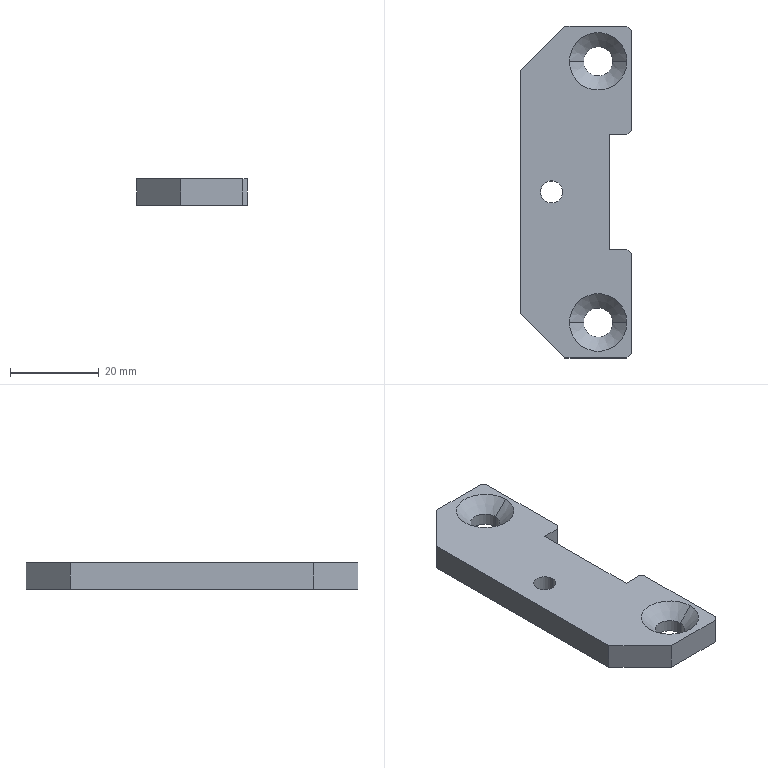Part | SolidWorks | features Chamfer 3, HoleWzd 2, ExtruThin 1, ICE 1 | 1 solid | 26 faces | box 25 x 75 x 6 mm | volume 9049 mm3 | plane 16 | cylinder 6 | cone 4 | commonest cylinder face diameters 6.6 x4 5 x2
STEP:
#1=CARTESIAN_POINT('',(-20.5,37.5,0.));
#2=VERTEX_POINT('',#1);
#3=CARTESIAN_POINT('',(-15.5,37.5,0.));
#4=VERTEX_POINT('',#3);
#5=CARTESIAN_POINT('',(-18.,37.5,0.));
#6=DIRECTION('',(0.,0.,1.));
#7=DIRECTION('',(1.,0.,0.));
#8=AXIS2_PLACEMENT_3D('',#5,#6,#7);
#9=CIRCLE('',#8,2.5);
#10=EDGE_CURVE('',#2,#4,#9,.T.);
#11=ORIENTED_EDGE('',*,*,#10,.F.);
#12=CARTESIAN_POINT('',(-20.5,37.5,6.));
#13=VERTEX_POINT('',#12);
#14=CARTESIAN_POINT('',(-20.5,37.5,6.));
#15=DIRECTION('',(0.,0.,1.));
#16=VECTOR('',#15,1000.);
#17=LINE('',#14,#16);
#18=EDGE_CURVE('',#2,#13,#17,.T.);
#19=ORIENTED_EDGE('',*,*,#18,.T.);
#20=CARTESIAN_POINT('',(-15.5,37.5,6.));
#21=VERTEX_POINT('',#20);
#22=CARTESIAN_POINT('',(-18.,37.5,6.));
#23=DIRECTION('',(0.,0.,1.));
#24=DIRECTION('',(1.,0.,0.));
#25=AXIS2_PLACEMENT_3D('',#22,#23,#24);
#26=CIRCLE('',#25,2.5);
#27=EDGE_CURVE('',#13,#21,#26,.T.);
#28=ORIENTED_EDGE('',*,*,#27,.T.);
#29=CARTESIAN_POINT('',(-15.5,37.5,6.));
#30=DIRECTION('',(0.,0.,1.));
#31=VECTOR('',#30,1000.);
#32=LINE('',#29,#31);
#33=EDGE_CURVE('',#4,#21,#32,.T.);
#34=ORIENTED_EDGE('',*,*,#33,.F.);
#35=EDGE_LOOP('',(#11,#19,#28,#34));
#36=FACE_OUTER_BOUND('',#35,.T.);
#37=CARTESIAN_POINT('',(-18.,37.5,6.));
#38=DIRECTION('',(0.,0.,1.));
#39=DIRECTION('',(1.,0.,0.));
#40=AXIS2_PLACEMENT_3D('',#37,#38,#39);
#41=CYLINDRICAL_SURFACE('',#40,2.5);
#42=ADVANCED_FACE('',(#36),#41,.F.);
#43=CARTESIAN_POINT('',(-10.8,67.,2.8));
#44=VERTEX_POINT('',#43);
#45=CARTESIAN_POINT('',(-4.2,67.,2.8));
#46=VERTEX_POINT('',#45);
#47=CARTESIAN_POINT('',(-7.5,67.,2.8));
#48=DIRECTION('',(0.,0.,1.));
#49=DIRECTION('',(1.,0.,0.));
#50=AXIS2_PLACEMENT_3D('',#47,#48,#49);
#51=CIRCLE('',#50,3.3);
#52=EDGE_CURVE('',#44,#46,#51,.T.);
#53=ORIENTED_EDGE('',*,*,#52,.F.);
#54=CARTESIAN_POINT('',(-14.,67.,6.));
#55=VERTEX_POINT('',#54);
#56=CARTESIAN_POINT('',(-14.,67.,6.));
#57=DIRECTION('',(-0.7071,0.,0.7071));
#58=VECTOR('',#57,1000.);
#59=LINE('',#56,#58);
#60=EDGE_CURVE('',#44,#55,#59,.T.);
#61=ORIENTED_EDGE('',*,*,#60,.T.);
#62=CARTESIAN_POINT('',(-1.,67.,6.));
#63=VERTEX_POINT('',#62);
#64=CARTESIAN_POINT('',(-7.5,67.,6.));
#65=DIRECTION('',(0.,0.,1.));
#66=DIRECTION('',(1.,0.,0.));
#67=AXIS2_PLACEMENT_3D('',#64,#65,#66);
#68=CIRCLE('',#67,6.5);
#69=EDGE_CURVE('',#55,#63,#68,.T.);
#70=ORIENTED_EDGE('',*,*,#69,.T.);
#71=CARTESIAN_POINT('',(-1.,67.,6.));
#72=DIRECTION('',(0.7071,0.,0.7071));
#73=VECTOR('',#72,1000.);
#74=LINE('',#71,#73);
#75=EDGE_CURVE('',#46,#63,#74,.T.);
#76=ORIENTED_EDGE('',*,*,#75,.F.);
#77=EDGE_LOOP('',(#53,#61,#70,#76));
#78=FACE_OUTER_BOUND('',#77,.T.);
#79=CARTESIAN_POINT('',(-7.5,67.,6.));
#80=DIRECTION('',(0.,0.,1.));
#81=DIRECTION('',(1.,0.,0.));
#82=AXIS2_PLACEMENT_3D('',#79,#80,#81);
#83=CONICAL_SURFACE('',#82,6.5,0.7854);
#84=ADVANCED_FACE('',(#78),#83,.F.);
#85=CARTESIAN_POINT('',(-10.8,67.,0.));
#86=VERTEX_POINT('',#85);
#87=CARTESIAN_POINT('',(-4.2,67.,0.));
#88=VERTEX_POINT('',#87);
#89=CARTESIAN_POINT('',(-7.5,67.,0.));
#90=DIRECTION('',(0.,0.,1.));
#91=DIRECTION('',(1.,0.,0.));
#92=AXIS2_PLACEMENT_3D('',#89,#90,#91);
#93=CIRCLE('',#92,3.3);
#94=EDGE_CURVE('',#86,#88,#93,.T.);
#95=ORIENTED_EDGE('',*,*,#94,.F.);
#96=CARTESIAN_POINT('',(-10.8,67.,6.));
#97=DIRECTION('',(0.,0.,1.));
#98=VECTOR('',#97,1000.);
#99=LINE('',#96,#98);
#100=EDGE_CURVE('',#86,#44,#99,.T.);
#101=ORIENTED_EDGE('',*,*,#100,.T.);
#102=ORIENTED_EDGE('',*,*,#52,.T.);
#103=CARTESIAN_POINT('',(-4.2,67.,6.));
#104=DIRECTION('',(0.,0.,1.));
#105=VECTOR('',#104,1000.);
#106=LINE('',#103,#105);
#107=EDGE_CURVE('',#88,#46,#106,.T.);
#108=ORIENTED_EDGE('',*,*,#107,.F.);
#109=EDGE_LOOP('',(#95,#101,#102,#108));
#110=FACE_OUTER_BOUND('',#109,.T.);
#111=CARTESIAN_POINT('',(-7.5,67.,6.));
#112=DIRECTION('',(0.,0.,1.));
#113=DIRECTION('',(1.,0.,0.));
#114=AXIS2_PLACEMENT_3D('',#111,#112,#113);
#115=CYLINDRICAL_SURFACE('',#114,3.3);
#116=ADVANCED_FACE('',(#110),#115,.F.);
#117=CARTESIAN_POINT('',(-10.8,8.,2.8));
#118=VERTEX_POINT('',#117);
#119=CARTESIAN_POINT('',(-4.2,8.,2.8));
#120=VERTEX_POINT('',#119);
#121=CARTESIAN_POINT('',(-7.5,8.,2.8));
#122=DIRECTION('',(0.,0.,1.));
#123=DIRECTION('',(1.,0.,0.));
#124=AXIS2_PLACEMENT_3D('',#121,#122,#123);
#125=CIRCLE('',#124,3.3);
#126=EDGE_CURVE('',#118,#120,#125,.T.);
#127=ORIENTED_EDGE('',*,*,#126,.F.);
#128=CARTESIAN_POINT('',(-14.,8.,6.));
#129=VERTEX_POINT('',#128);
#130=CARTESIAN_POINT('',(-14.,8.,6.));
#131=DIRECTION('',(-0.7071,0.,0.7071));
#132=VECTOR('',#131,1000.);
#133=LINE('',#130,#132);
#134=EDGE_CURVE('',#118,#129,#133,.T.);
#135=ORIENTED_EDGE('',*,*,#134,.T.);
#136=CARTESIAN_POINT('',(-1.,8.,6.));
#137=VERTEX_POINT('',#136);
#138=CARTESIAN_POINT('',(-7.5,8.,6.));
#139=DIRECTION('',(0.,0.,1.));
#140=DIRECTION('',(1.,0.,0.));
#141=AXIS2_PLACEMENT_3D('',#138,#139,#140);
#142=CIRCLE('',#141,6.5);
#143=EDGE_CURVE('',#129,#137,#142,.T.);
#144=ORIENTED_EDGE('',*,*,#143,.T.);
#145=CARTESIAN_POINT('',(-1.,8.,6.));
#146=DIRECTION('',(0.7071,0.,0.7071));
#147=VECTOR('',#146,1000.);
#148=LINE('',#145,#147);
#149=EDGE_CURVE('',#120,#137,#148,.T.);
#150=ORIENTED_EDGE('',*,*,#149,.F.);
#151=EDGE_LOOP('',(#127,#135,#144,#150));
#152=FACE_OUTER_BOUND('',#151,.T.);
#153=CARTESIAN_POINT('',(-7.5,8.,6.));
#154=DIRECTION('',(0.,0.,1.));
#155=DIRECTION('',(1.,0.,0.));
#156=AXIS2_PLACEMENT_3D('',#153,#154,#155);
#157=CONICAL_SURFACE('',#156,6.5,0.7854);
#158=ADVANCED_FACE('',(#152),#157,.F.);
#159=CARTESIAN_POINT('',(-10.8,8.,0.));
#160=VERTEX_POINT('',#159);
#161=CARTESIAN_POINT('',(-4.2,8.,0.));
#162=VERTEX_POINT('',#161);
#163=CARTESIAN_POINT('',(-7.5,8.,0.));
#164=DIRECTION('',(0.,0.,1.));
#165=DIRECTION('',(1.,0.,0.));
#166=AXIS2_PLACEMENT_3D('',#163,#164,#165);
#167=CIRCLE('',#166,3.3);
#168=EDGE_CURVE('',#160,#162,#167,.T.);
#169=ORIENTED_EDGE('',*,*,#168,.F.);
#170=CARTESIAN_POINT('',(-10.8,8.,6.));
#171=DIRECTION('',(0.,0.,1.));
#172=VECTOR('',#171,1000.);
#173=LINE('',#170,#172);
#174=EDGE_CURVE('',#160,#118,#173,.T.);
#175=ORIENTED_EDGE('',*,*,#174,.T.);
#176=ORIENTED_EDGE('',*,*,#126,.T.);
#177=CARTESIAN_POINT('',(-4.2,8.,6.));
#178=DIRECTION('',(0.,0.,1.));
#179=VECTOR('',#178,1000.);
#180=LINE('',#177,#179);
#181=EDGE_CURVE('',#162,#120,#180,.T.);
#182=ORIENTED_EDGE('',*,*,#181,.F.);
#183=EDGE_LOOP('',(#169,#175,#176,#182));
#184=FACE_OUTER_BOUND('',#183,.T.);
#185=CARTESIAN_POINT('',(-7.5,8.,6.));
#186=DIRECTION('',(0.,0.,1.));
#187=DIRECTION('',(1.,0.,0.));
#188=AXIS2_PLACEMENT_3D('',#185,#186,#187);
#189=CYLINDRICAL_SURFACE('',#188,3.3);
#190=ADVANCED_FACE('',(#184),#189,.F.);
#191=CARTESIAN_POINT('',(0.,74.,6.));
#192=VERTEX_POINT('',#191);
#193=CARTESIAN_POINT('',(0.,51.5,6.));
#194=VERTEX_POINT('',#193);
#195=CARTESIAN_POINT('',(0.,75.,6.));
#196=DIRECTION('',(0.,-1.,0.));
#197=VECTOR('',#196,1000.);
#198=LINE('',#195,#197);
#199=EDGE_CURVE('',#192,#194,#198,.T.);
#200=ORIENTED_EDGE('',*,*,#199,.T.);
#201=CARTESIAN_POINT('',(0.,51.5,0.));
#202=VERTEX_POINT('',#201);
#203=CARTESIAN_POINT('',(0.,51.5,0.));
#204=DIRECTION('',(0.,0.,-1.));
#205=VECTOR('',#204,1000.);
#206=LINE('',#203,#205);
#207=EDGE_CURVE('',#194,#202,#206,.T.);
#208=ORIENTED_EDGE('',*,*,#207,.T.);
#209=CARTESIAN_POINT('',(0.,74.,0.));
#210=VERTEX_POINT('',#209);
#211=CARTESIAN_POINT('',(0.,75.,0.));
#212=DIRECTION('',(0.,-1.,0.));
#213=VECTOR('',#212,1000.);
#214=LINE('',#211,#213);
#215=EDGE_CURVE('',#210,#202,#214,.T.);
#216=ORIENTED_EDGE('',*,*,#215,.F.);
#217=CARTESIAN_POINT('',(0.,74.,6.));
#218=DIRECTION('',(0.,0.,1.));
#219=VECTOR('',#218,1000.);
#220=LINE('',#217,#219);
#221=EDGE_CURVE('',#210,#192,#220,.T.);
#222=ORIENTED_EDGE('',*,*,#221,.T.);
#223=EDGE_LOOP('',(#200,#208,#216,#222));
#224=FACE_OUTER_BOUND('',#223,.T.);
#225=CARTESIAN_POINT('',(0.,75.,6.));
#226=DIRECTION('',(1.,0.,0.));
#227=DIRECTION('',(0.,1.,0.));
#228=AXIS2_PLACEMENT_3D('',#225,#226,#227);
#229=PLANE('',#228);
#230=ADVANCED_FACE('',(#224),#229,.T.);
#231=CARTESIAN_POINT('',(-25.,65.,0.));
#232=VERTEX_POINT('',#231);
#233=CARTESIAN_POINT('',(-25.,10.,0.));
#234=VERTEX_POINT('',#233);
#235=CARTESIAN_POINT('',(-25.,75.,0.));
#236=DIRECTION('',(0.,-1.,0.));
#237=VECTOR('',#236,1000.);
#238=LINE('',#235,#237);
#239=EDGE_CURVE('',#232,#234,#238,.T.);
#240=ORIENTED_EDGE('',*,*,#239,.T.);
#241=CARTESIAN_POINT('',(-25.,10.,6.));
#242=VERTEX_POINT('',#241);
#243=CARTESIAN_POINT('',(-25.,10.,6.));
#244=DIRECTION('',(0.,0.,1.));
#245=VECTOR('',#244,1000.);
#246=LINE('',#243,#245);
#247=EDGE_CURVE('',#234,#242,#246,.T.);
#248=ORIENTED_EDGE('',*,*,#247,.T.);
#249=CARTESIAN_POINT('',(-25.,65.,6.));
#250=VERTEX_POINT('',#249);
#251=CARTESIAN_POINT('',(-25.,75.,6.));
#252=DIRECTION('',(0.,-1.,0.));
#253=VECTOR('',#252,1000.);
#254=LINE('',#251,#253);
#255=EDGE_CURVE('',#250,#242,#254,.T.);
#256=ORIENTED_EDGE('',*,*,#255,.F.);
#257=CARTESIAN_POINT('',(-25.,65.,0.));
#258=DIRECTION('',(0.,0.,-1.));
#259=VECTOR('',#258,1000.);
#260=LINE('',#257,#259);
#261=EDGE_CURVE('',#250,#232,#260,.T.);
#262=ORIENTED_EDGE('',*,*,#261,.T.);
#263=EDGE_LOOP('',(#240,#248,#256,#262));
#264=FACE_OUTER_BOUND('',#263,.T.);
#265=CARTESIAN_POINT('',(-25.,75.,6.));
#266=DIRECTION('',(1.,0.,0.));
#267=DIRECTION('',(0.,1.,0.));
#268=AXIS2_PLACEMENT_3D('',#265,#266,#267);
#269=PLANE('',#268);
#270=ADVANCED_FACE('',(#264),#269,.F.);
#271=CARTESIAN_POINT('',(-1.,0.,6.));
#272=VERTEX_POINT('',#271);
#273=CARTESIAN_POINT('',(-15.,0.,6.));
#274=VERTEX_POINT('',#273);
#275=CARTESIAN_POINT('',(0.,0.,6.));
#276=DIRECTION('',(-1.,0.,0.));
#277=VECTOR('',#276,1000.);
#278=LINE('',#275,#277);
#279=EDGE_CURVE('',#272,#274,#278,.T.);
#280=ORIENTED_EDGE('',*,*,#279,.T.);
#281=CARTESIAN_POINT('',(-15.,0.,0.));
#282=VERTEX_POINT('',#281);
#283=CARTESIAN_POINT('',(-15.,0.,0.));
#284=DIRECTION('',(0.,0.,-1.));
#285=VECTOR('',#284,1000.);
#286=LINE('',#283,#285);
#287=EDGE_CURVE('',#274,#282,#286,.T.);
#288=ORIENTED_EDGE('',*,*,#287,.T.);
#289=CARTESIAN_POINT('',(-1.,0.,0.));
#290=VERTEX_POINT('',#289);
#291=CARTESIAN_POINT('',(0.,0.,0.));
#292=DIRECTION('',(-1.,0.,0.));
#293=VECTOR('',#292,1000.);
#294=LINE('',#291,#293);
#295=EDGE_CURVE('',#290,#282,#294,.T.);
#296=ORIENTED_EDGE('',*,*,#295,.F.);
#297=CARTESIAN_POINT('',(-1.,0.,6.));
#298=DIRECTION('',(0.,0.,1.));
#299=VECTOR('',#298,1000.);
#300=LINE('',#297,#299);
#301=EDGE_CURVE('',#290,#272,#300,.T.);
#302=ORIENTED_EDGE('',*,*,#301,.T.);
#303=EDGE_LOOP('',(#280,#288,#296,#302));
#304=FACE_OUTER_BOUND('',#303,.T.);
#305=CARTESIAN_POINT('',(0.,0.,6.));
#306=DIRECTION('',(0.,-1.,0.));
#307=DIRECTION('',(0.,0.,-1.));
#308=AXIS2_PLACEMENT_3D('',#305,#306,#307);
#309=PLANE('',#308);
#310=ADVANCED_FACE('',(#304),#309,.T.);
#311=CARTESIAN_POINT('',(0.,23.5,0.));
#312=VERTEX_POINT('',#311);
#313=CARTESIAN_POINT('',(0.,1.,0.));
#314=VERTEX_POINT('',#313);
#315=CARTESIAN_POINT('',(0.,75.,0.));
#316=DIRECTION('',(0.,-1.,0.));
#317=VECTOR('',#316,1000.);
#318=LINE('',#315,#317);
#319=EDGE_CURVE('',#312,#314,#318,.T.);
#320=ORIENTED_EDGE('',*,*,#319,.F.);
#321=CARTESIAN_POINT('',(0.,23.5,6.));
#322=VERTEX_POINT('',#321);
#323=CARTESIAN_POINT('',(0.,23.5,6.));
#324=DIRECTION('',(0.,0.,1.));
#325=VECTOR('',#324,1000.);
#326=LINE('',#323,#325);
#327=EDGE_CURVE('',#312,#322,#326,.T.);
#328=ORIENTED_EDGE('',*,*,#327,.T.);
#329=CARTESIAN_POINT('',(0.,1.,6.));
#330=VERTEX_POINT('',#329);
#331=CARTESIAN_POINT('',(0.,75.,6.));
#332=DIRECTION('',(0.,-1.,0.));
#333=VECTOR('',#332,1000.);
#334=LINE('',#331,#333);
#335=EDGE_CURVE('',#322,#330,#334,.T.);
#336=ORIENTED_EDGE('',*,*,#335,.T.);
#337=CARTESIAN_POINT('',(0.,1.,6.));
#338=DIRECTION('',(0.,0.,-1.));
#339=VECTOR('',#338,1000.);
#340=LINE('',#337,#339);
#341=EDGE_CURVE('',#330,#314,#340,.T.);
#342=ORIENTED_EDGE('',*,*,#341,.T.);
#343=EDGE_LOOP('',(#320,#328,#336,#342));
#344=FACE_OUTER_BOUND('',#343,.T.);
#345=CARTESIAN_POINT('',(0.,75.,6.));
#346=DIRECTION('',(1.,0.,0.));
#347=DIRECTION('',(0.,1.,0.));
#348=AXIS2_PLACEMENT_3D('',#345,#346,#347);
#349=PLANE('',#348);
#350=ADVANCED_FACE('',(#344),#349,.T.);
#351=CARTESIAN_POINT('',(-15.,75.,0.));
#352=VERTEX_POINT('',#351);
#353=CARTESIAN_POINT('',(-1.,75.,0.));
#354=VERTEX_POINT('',#353);
#355=CARTESIAN_POINT('',(-25.,75.,0.));
#356=DIRECTION('',(1.,0.,0.));
#357=VECTOR('',#356,1000.);
#358=LINE('',#355,#357);
#359=EDGE_CURVE('',#352,#354,#358,.T.);
#360=ORIENTED_EDGE('',*,*,#359,.F.);
#361=CARTESIAN_POINT('',(-15.,75.,6.));
#362=VERTEX_POINT('',#361);
#363=CARTESIAN_POINT('',(-15.,75.,6.));
#364=DIRECTION('',(0.,0.,1.));
#365=VECTOR('',#364,1000.);
#366=LINE('',#363,#365);
#367=EDGE_CURVE('',#352,#362,#366,.T.);
#368=ORIENTED_EDGE('',*,*,#367,.T.);
#369=CARTESIAN_POINT('',(-1.,75.,6.));
#370=VERTEX_POINT('',#369);
#371=CARTESIAN_POINT('',(-25.,75.,6.));
#372=DIRECTION('',(1.,0.,0.));
#373=VECTOR('',#372,1000.);
#374=LINE('',#371,#373);
#375=EDGE_CURVE('',#362,#370,#374,.T.);
#376=ORIENTED_EDGE('',*,*,#375,.T.);
#377=CARTESIAN_POINT('',(-1.,75.,6.));
#378=DIRECTION('',(0.,0.,-1.));
#379=VECTOR('',#378,1000.);
#380=LINE('',#377,#379);
#381=EDGE_CURVE('',#370,#354,#380,.T.);
#382=ORIENTED_EDGE('',*,*,#381,.T.);
#383=EDGE_LOOP('',(#360,#368,#376,#382));
#384=FACE_OUTER_BOUND('',#383,.T.);
#385=CARTESIAN_POINT('',(-25.,75.,6.));
#386=DIRECTION('',(0.,1.,0.));
#387=DIRECTION('',(0.,0.,1.));
#388=AXIS2_PLACEMENT_3D('',#385,#386,#387);
#389=PLANE('',#388);
#390=ADVANCED_FACE('',(#384),#389,.T.);
#391=CARTESIAN_POINT('',(-18.,37.5,6.));
#392=DIRECTION('',(0.,0.,1.));
#393=DIRECTION('',(1.,0.,0.));
#394=AXIS2_PLACEMENT_3D('',#391,#392,#393);
#395=CIRCLE('',#394,2.5);
#396=EDGE_CURVE('',#21,#13,#395,.T.);
#397=ORIENTED_EDGE('',*,*,#396,.F.);
#398=ORIENTED_EDGE('',*,*,#27,.F.);
#399=EDGE_LOOP('',(#397,#398));
#400=FACE_BOUND('',#399,.T.);
#401=CARTESIAN_POINT('',(-7.5,67.,6.));
#402=DIRECTION('',(0.,0.,1.));
#403=DIRECTION('',(1.,0.,0.));
#404=AXIS2_PLACEMENT_3D('',#401,#402,#403);
#405=CIRCLE('',#404,6.5);
#406=EDGE_CURVE('',#63,#55,#405,.T.);
#407=ORIENTED_EDGE('',*,*,#406,.F.);
#408=ORIENTED_EDGE('',*,*,#69,.F.);
#409=EDGE_LOOP('',(#407,#408));
#410=FACE_BOUND('',#409,.T.);
#411=CARTESIAN_POINT('',(-7.5,8.,6.));
#412=DIRECTION('',(0.,0.,1.));
#413=DIRECTION('',(1.,0.,0.));
#414=AXIS2_PLACEMENT_3D('',#411,#412,#413);
#415=CIRCLE('',#414,6.5);
#416=EDGE_CURVE('',#137,#129,#415,.T.);
#417=ORIENTED_EDGE('',*,*,#416,.F.);
#418=ORIENTED_EDGE('',*,*,#143,.F.);
#419=EDGE_LOOP('',(#417,#418));
#420=FACE_BOUND('',#419,.T.);
#421=ORIENTED_EDGE('',*,*,#335,.F.);
#422=CARTESIAN_POINT('',(-1.,24.5,6.));
#423=VERTEX_POINT('',#422);
#424=CARTESIAN_POINT('',(-1.,24.5,6.));
#425=DIRECTION('',(-0.7071,0.7071,0.));
#426=VECTOR('',#425,1000.);
#427=LINE('',#424,#426);
#428=EDGE_CURVE('',#322,#423,#427,.T.);
#429=ORIENTED_EDGE('',*,*,#428,.T.);
#430=CARTESIAN_POINT('',(-5.,24.5,6.));
#431=VERTEX_POINT('',#430);
#432=CARTESIAN_POINT('',(15.259,24.5,6.));
#433=DIRECTION('',(1.,0.,0.));
#434=VECTOR('',#433,1000.);
#435=LINE('',#432,#434);
#436=EDGE_CURVE('',#431,#423,#435,.T.);
#437=ORIENTED_EDGE('',*,*,#436,.F.);
#438=CARTESIAN_POINT('',(-5.,50.5,6.));
#439=VERTEX_POINT('',#438);
#440=CARTESIAN_POINT('',(-5.,50.5,6.));
#441=DIRECTION('',(0.,-1.,0.));
#442=VECTOR('',#441,1000.);
#443=LINE('',#440,#442);
#444=EDGE_CURVE('',#439,#431,#443,.T.);
#445=ORIENTED_EDGE('',*,*,#444,.F.);
#446=CARTESIAN_POINT('',(-1.,50.5,6.));
#447=VERTEX_POINT('',#446);
#448=CARTESIAN_POINT('',(15.259,50.5,6.));
#449=DIRECTION('',(-1.,0.,0.));
#450=VECTOR('',#449,1000.);
#451=LINE('',#448,#450);
#452=EDGE_CURVE('',#447,#439,#451,.T.);
#453=ORIENTED_EDGE('',*,*,#452,.F.);
#454=CARTESIAN_POINT('',(-1.,50.5,6.));
#455=DIRECTION('',(0.7071,0.7071,0.));
#456=VECTOR('',#455,1000.);
#457=LINE('',#454,#456);
#458=EDGE_CURVE('',#447,#194,#457,.T.);
#459=ORIENTED_EDGE('',*,*,#458,.T.);
#460=ORIENTED_EDGE('',*,*,#199,.F.);
#461=CARTESIAN_POINT('',(-1.,75.,6.));
#462=DIRECTION('',(-0.7071,0.7071,0.));
#463=VECTOR('',#462,1000.);
#464=LINE('',#461,#463);
#465=EDGE_CURVE('',#192,#370,#464,.T.);
#466=ORIENTED_EDGE('',*,*,#465,.T.);
#467=ORIENTED_EDGE('',*,*,#375,.F.);
#468=CARTESIAN_POINT('',(-25.,65.,6.));
#469=DIRECTION('',(-0.7071,-0.7071,0.));
#470=VECTOR('',#469,1000.);
#471=LINE('',#468,#470);
#472=EDGE_CURVE('',#362,#250,#471,.T.);
#473=ORIENTED_EDGE('',*,*,#472,.T.);
#474=ORIENTED_EDGE('',*,*,#255,.T.);
#475=CARTESIAN_POINT('',(-15.,0.,6.));
#476=DIRECTION('',(0.7071,-0.7071,0.));
#477=VECTOR('',#476,1000.);
#478=LINE('',#475,#477);
#479=EDGE_CURVE('',#242,#274,#478,.T.);
#480=ORIENTED_EDGE('',*,*,#479,.T.);
#481=ORIENTED_EDGE('',*,*,#279,.F.);
#482=CARTESIAN_POINT('',(0.,1.,6.));
#483=DIRECTION('',(0.7071,0.7071,0.));
#484=VECTOR('',#483,1000.);
#485=LINE('',#482,#484);
#486=EDGE_CURVE('',#272,#330,#485,.T.);
#487=ORIENTED_EDGE('',*,*,#486,.T.);
#488=EDGE_LOOP('',(#421,#429,#437,#445,#453,#459,#460,#466,#467,#473,#474,#480,#481,#487));
#489=FACE_OUTER_BOUND('',#488,.T.);
#490=CARTESIAN_POINT('',(0.,0.,6.));
#491=DIRECTION('',(0.,0.,-1.));
#492=DIRECTION('',(-1.,0.,0.));
#493=AXIS2_PLACEMENT_3D('',#490,#491,#492);
#494=PLANE('',#493);
#495=ADVANCED_FACE('',(#400,#410,#420,#489),#494,.F.);
#496=CARTESIAN_POINT('',(-1.,24.5,0.));
#497=VERTEX_POINT('',#496);
#498=CARTESIAN_POINT('',(-5.,24.5,0.));
#499=VERTEX_POINT('',#498);
#500=CARTESIAN_POINT('',(0.,24.5,0.));
#501=DIRECTION('',(-1.,0.,0.));
#502=VECTOR('',#501,1000.);
#503=LINE('',#500,#502);
#504=EDGE_CURVE('',#497,#499,#503,.T.);
#505=ORIENTED_EDGE('',*,*,#504,.F.);
#506=CARTESIAN_POINT('',(11.75,11.75,0.));
#507=DIRECTION('',(0.7071,-0.7071,0.));
#508=VECTOR('',#507,1000.);
#509=LINE('',#506,#508);
#510=EDGE_CURVE('',#497,#312,#509,.T.);
#511=ORIENTED_EDGE('',*,*,#510,.T.);
#512=ORIENTED_EDGE('',*,*,#319,.T.);
#513=CARTESIAN_POINT('',(-0.5,0.5,0.));
#514=DIRECTION('',(-0.7071,-0.7071,0.));
#515=VECTOR('',#514,1000.);
#516=LINE('',#513,#515);
#517=EDGE_CURVE('',#314,#290,#516,.T.);
#518=ORIENTED_EDGE('',*,*,#517,.T.);
#519=ORIENTED_EDGE('',*,*,#295,.T.);
#520=CARTESIAN_POINT('',(-7.5,-7.5,0.));
#521=DIRECTION('',(-0.7071,0.7071,0.));
#522=VECTOR('',#521,1000.);
#523=LINE('',#520,#522);
#524=EDGE_CURVE('',#282,#234,#523,.T.);
#525=ORIENTED_EDGE('',*,*,#524,.T.);
#526=ORIENTED_EDGE('',*,*,#239,.F.);
#527=CARTESIAN_POINT('',(-45.,45.,0.));
#528=DIRECTION('',(0.7071,0.7071,0.));
#529=VECTOR('',#528,1000.);
#530=LINE('',#527,#529);
#531=EDGE_CURVE('',#232,#352,#530,.T.);
#532=ORIENTED_EDGE('',*,*,#531,.T.);
#533=ORIENTED_EDGE('',*,*,#359,.T.);
#534=CARTESIAN_POINT('',(37.,37.,0.));
#535=DIRECTION('',(0.7071,-0.7071,0.));
#536=VECTOR('',#535,1000.);
#537=LINE('',#534,#536);
#538=EDGE_CURVE('',#354,#210,#537,.T.);
#539=ORIENTED_EDGE('',*,*,#538,.T.);
#540=ORIENTED_EDGE('',*,*,#215,.T.);
#541=CARTESIAN_POINT('',(-1.,50.5,0.));
#542=VERTEX_POINT('',#541);
#543=CARTESIAN_POINT('',(-25.75,25.75,0.));
#544=DIRECTION('',(-0.7071,-0.7071,0.));
#545=VECTOR('',#544,1000.);
#546=LINE('',#543,#545);
#547=EDGE_CURVE('',#202,#542,#546,.T.);
#548=ORIENTED_EDGE('',*,*,#547,.T.);
#549=CARTESIAN_POINT('',(-5.,50.5,0.));
#550=VERTEX_POINT('',#549);
#551=CARTESIAN_POINT('',(0.,50.5,0.));
#552=DIRECTION('',(1.,0.,0.));
#553=VECTOR('',#552,1000.);
#554=LINE('',#551,#553);
#555=EDGE_CURVE('',#550,#542,#554,.T.);
#556=ORIENTED_EDGE('',*,*,#555,.F.);
#557=CARTESIAN_POINT('',(-5.,0.,0.));
#558=DIRECTION('',(0.,1.,0.));
#559=VECTOR('',#558,1000.);
#560=LINE('',#557,#559);
#561=EDGE_CURVE('',#499,#550,#560,.T.);
#562=ORIENTED_EDGE('',*,*,#561,.F.);
#563=EDGE_LOOP('',(#505,#511,#512,#518,#519,#525,#526,#532,#533,#539,#540,#548,#556,#562));
#564=FACE_OUTER_BOUND('',#563,.T.);
#565=CARTESIAN_POINT('',(-18.,37.5,0.));
#566=DIRECTION('',(0.,0.,1.));
#567=DIRECTION('',(1.,0.,0.));
#568=AXIS2_PLACEMENT_3D('',#565,#566,#567);
#569=CIRCLE('',#568,2.5);
#570=EDGE_CURVE('',#4,#2,#569,.T.);
#571=ORIENTED_EDGE('',*,*,#570,.T.);
#572=ORIENTED_EDGE('',*,*,#10,.T.);
#573=EDGE_LOOP('',(#571,#572));
#574=FACE_BOUND('',#573,.T.);
#575=CARTESIAN_POINT('',(-7.5,67.,0.));
#576=DIRECTION('',(0.,0.,1.));
#577=DIRECTION('',(1.,0.,0.));
#578=AXIS2_PLACEMENT_3D('',#575,#576,#577);
#579=CIRCLE('',#578,3.3);
#580=EDGE_CURVE('',#88,#86,#579,.T.);
#581=ORIENTED_EDGE('',*,*,#580,.T.);
#582=ORIENTED_EDGE('',*,*,#94,.T.);
#583=EDGE_LOOP('',(#581,#582));
#584=FACE_BOUND('',#583,.T.);
#585=CARTESIAN_POINT('',(-7.5,8.,0.));
#586=DIRECTION('',(0.,0.,1.));
#587=DIRECTION('',(1.,0.,0.));
#588=AXIS2_PLACEMENT_3D('',#585,#586,#587);
#589=CIRCLE('',#588,3.3);
#590=EDGE_CURVE('',#162,#160,#589,.T.);
#591=ORIENTED_EDGE('',*,*,#590,.T.);
#592=ORIENTED_EDGE('',*,*,#168,.T.);
#593=EDGE_LOOP('',(#591,#592));
#594=FACE_BOUND('',#593,.T.);
#595=CARTESIAN_POINT('',(0.,0.,0.));
#596=DIRECTION('',(0.,0.,-1.));
#597=DIRECTION('',(-1.,0.,0.));
#598=AXIS2_PLACEMENT_3D('',#595,#596,#597);
#599=PLANE('',#598);
#600=ADVANCED_FACE('',(#564,#574,#584,#594),#599,.T.);
#601=ORIENTED_EDGE('',*,*,#465,.F.);
#602=ORIENTED_EDGE('',*,*,#221,.F.);
#603=ORIENTED_EDGE('',*,*,#538,.F.);
#604=ORIENTED_EDGE('',*,*,#381,.F.);
#605=EDGE_LOOP('',(#601,#602,#603,#604));
#606=FACE_OUTER_BOUND('',#605,.T.);
#607=CARTESIAN_POINT('',(-1.,75.,6.));
#608=DIRECTION('',(-0.7071,-0.7071,0.));
#609=DIRECTION('',(0.,0.,-1.));
#610=AXIS2_PLACEMENT_3D('',#607,#608,#609);
#611=PLANE('',#610);
#612=ADVANCED_FACE('',(#606),#611,.F.);
#613=ORIENTED_EDGE('',*,*,#486,.F.);
#614=ORIENTED_EDGE('',*,*,#301,.F.);
#615=ORIENTED_EDGE('',*,*,#517,.F.);
#616=ORIENTED_EDGE('',*,*,#341,.F.);
#617=EDGE_LOOP('',(#613,#614,#615,#616));
#618=FACE_OUTER_BOUND('',#617,.T.);
#619=CARTESIAN_POINT('',(0.,1.,6.));
#620=DIRECTION('',(-0.7071,0.7071,0.));
#621=DIRECTION('',(0.,0.,-1.));
#622=AXIS2_PLACEMENT_3D('',#619,#620,#621);
#623=PLANE('',#622);
#624=ADVANCED_FACE('',(#618),#623,.F.);
#625=ORIENTED_EDGE('',*,*,#174,.F.);
#626=ORIENTED_EDGE('',*,*,#590,.F.);
#627=ORIENTED_EDGE('',*,*,#181,.T.);
#628=CARTESIAN_POINT('',(-7.5,8.,2.8));
#629=DIRECTION('',(0.,0.,1.));
#630=DIRECTION('',(1.,0.,0.));
#631=AXIS2_PLACEMENT_3D('',#628,#629,#630);
#632=CIRCLE('',#631,3.3);
#633=EDGE_CURVE('',#120,#118,#632,.T.);
#634=ORIENTED_EDGE('',*,*,#633,.T.);
#635=EDGE_LOOP('',(#625,#626,#627,#634));
#636=FACE_OUTER_BOUND('',#635,.T.);
#637=CARTESIAN_POINT('',(-7.5,8.,6.));
#638=DIRECTION('',(0.,0.,1.));
#639=DIRECTION('',(1.,0.,0.));
#640=AXIS2_PLACEMENT_3D('',#637,#638,#639);
#641=CYLINDRICAL_SURFACE('',#640,3.3);
#642=ADVANCED_FACE('',(#636),#641,.F.);
#643=ORIENTED_EDGE('',*,*,#134,.F.);
#644=ORIENTED_EDGE('',*,*,#633,.F.);
#645=ORIENTED_EDGE('',*,*,#149,.T.);
#646=ORIENTED_EDGE('',*,*,#416,.T.);
#647=EDGE_LOOP('',(#643,#644,#645,#646));
#648=FACE_OUTER_BOUND('',#647,.T.);
#649=CARTESIAN_POINT('',(-7.5,8.,6.));
#650=DIRECTION('',(0.,0.,1.));
#651=DIRECTION('',(1.,0.,0.));
#652=AXIS2_PLACEMENT_3D('',#649,#650,#651);
#653=CONICAL_SURFACE('',#652,6.5,0.7854);
#654=ADVANCED_FACE('',(#648),#653,.F.);
#655=ORIENTED_EDGE('',*,*,#100,.F.);
#656=ORIENTED_EDGE('',*,*,#580,.F.);
#657=ORIENTED_EDGE('',*,*,#107,.T.);
#658=CARTESIAN_POINT('',(-7.5,67.,2.8));
#659=DIRECTION('',(0.,0.,1.));
#660=DIRECTION('',(1.,0.,0.));
#661=AXIS2_PLACEMENT_3D('',#658,#659,#660);
#662=CIRCLE('',#661,3.3);
#663=EDGE_CURVE('',#46,#44,#662,.T.);
#664=ORIENTED_EDGE('',*,*,#663,.T.);
#665=EDGE_LOOP('',(#655,#656,#657,#664));
#666=FACE_OUTER_BOUND('',#665,.T.);
#667=CARTESIAN_POINT('',(-7.5,67.,6.));
#668=DIRECTION('',(0.,0.,1.));
#669=DIRECTION('',(1.,0.,0.));
#670=AXIS2_PLACEMENT_3D('',#667,#668,#669);
#671=CYLINDRICAL_SURFACE('',#670,3.3);
#672=ADVANCED_FACE('',(#666),#671,.F.);
#673=ORIENTED_EDGE('',*,*,#60,.F.);
#674=ORIENTED_EDGE('',*,*,#663,.F.);
#675=ORIENTED_EDGE('',*,*,#75,.T.);
#676=ORIENTED_EDGE('',*,*,#406,.T.);
#677=EDGE_LOOP('',(#673,#674,#675,#676));
#678=FACE_OUTER_BOUND('',#677,.T.);
#679=CARTESIAN_POINT('',(-7.5,67.,6.));
#680=DIRECTION('',(0.,0.,1.));
#681=DIRECTION('',(1.,0.,0.));
#682=AXIS2_PLACEMENT_3D('',#679,#680,#681);
#683=CONICAL_SURFACE('',#682,6.5,0.7854);
#684=ADVANCED_FACE('',(#678),#683,.F.);
#685=ORIENTED_EDGE('',*,*,#479,.F.);
#686=ORIENTED_EDGE('',*,*,#247,.F.);
#687=ORIENTED_EDGE('',*,*,#524,.F.);
#688=ORIENTED_EDGE('',*,*,#287,.F.);
#689=EDGE_LOOP('',(#685,#686,#687,#688));
#690=FACE_OUTER_BOUND('',#689,.T.);
#691=CARTESIAN_POINT('',(-15.,0.,6.));
#692=DIRECTION('',(-0.7071,-0.7071,0.));
#693=DIRECTION('',(0.,0.,1.));
#694=AXIS2_PLACEMENT_3D('',#691,#692,#693);
#695=PLANE('',#694);
#696=ADVANCED_FACE('',(#690),#695,.T.);
#697=ORIENTED_EDGE('',*,*,#472,.F.);
#698=ORIENTED_EDGE('',*,*,#367,.F.);
#699=ORIENTED_EDGE('',*,*,#531,.F.);
#700=ORIENTED_EDGE('',*,*,#261,.F.);
#701=EDGE_LOOP('',(#697,#698,#699,#700));
#702=FACE_OUTER_BOUND('',#701,.T.);
#703=CARTESIAN_POINT('',(-25.,65.,6.));
#704=DIRECTION('',(-0.7071,0.7071,0.));
#705=DIRECTION('',(0.,0.,1.));
#706=AXIS2_PLACEMENT_3D('',#703,#704,#705);
#707=PLANE('',#706);
#708=ADVANCED_FACE('',(#702),#707,.T.);
#709=ORIENTED_EDGE('',*,*,#18,.F.);
#710=ORIENTED_EDGE('',*,*,#570,.F.);
#711=ORIENTED_EDGE('',*,*,#33,.T.);
#712=ORIENTED_EDGE('',*,*,#396,.T.);
#713=EDGE_LOOP('',(#709,#710,#711,#712));
#714=FACE_OUTER_BOUND('',#713,.T.);
#715=CARTESIAN_POINT('',(-18.,37.5,6.));
#716=DIRECTION('',(0.,0.,1.));
#717=DIRECTION('',(1.,0.,0.));
#718=AXIS2_PLACEMENT_3D('',#715,#716,#717);
#719=CYLINDRICAL_SURFACE('',#718,2.5);
#720=ADVANCED_FACE('',(#714),#719,.F.);
#721=ORIENTED_EDGE('',*,*,#561,.T.);
#722=CARTESIAN_POINT('',(-5.,50.5,-4.));
#723=DIRECTION('',(0.,0.,1.));
#724=VECTOR('',#723,1000.);
#725=LINE('',#722,#724);
#726=EDGE_CURVE('',#550,#439,#725,.T.);
#727=ORIENTED_EDGE('',*,*,#726,.T.);
#728=ORIENTED_EDGE('',*,*,#444,.T.);
#729=CARTESIAN_POINT('',(-5.,24.5,-4.));
#730=DIRECTION('',(0.,0.,1.));
#731=VECTOR('',#730,1000.);
#732=LINE('',#729,#731);
#733=EDGE_CURVE('',#499,#431,#732,.T.);
#734=ORIENTED_EDGE('',*,*,#733,.F.);
#735=EDGE_LOOP('',(#721,#727,#728,#734));
#736=FACE_OUTER_BOUND('',#735,.T.);
#737=CARTESIAN_POINT('',(-5.,50.5,-4.));
#738=DIRECTION('',(-1.,0.,0.));
#739=DIRECTION('',(0.,-1.,0.));
#740=AXIS2_PLACEMENT_3D('',#737,#738,#739);
#741=PLANE('',#740);
#742=ADVANCED_FACE('',(#736),#741,.F.);
#743=ORIENTED_EDGE('',*,*,#555,.T.);
#744=CARTESIAN_POINT('',(-1.,50.5,6.));
#745=DIRECTION('',(0.,0.,1.));
#746=VECTOR('',#745,1000.);
#747=LINE('',#744,#746);
#748=EDGE_CURVE('',#542,#447,#747,.T.);
#749=ORIENTED_EDGE('',*,*,#748,.T.);
#750=ORIENTED_EDGE('',*,*,#452,.T.);
#751=ORIENTED_EDGE('',*,*,#726,.F.);
#752=EDGE_LOOP('',(#743,#749,#750,#751));
#753=FACE_OUTER_BOUND('',#752,.T.);
#754=CARTESIAN_POINT('',(15.259,50.5,-4.));
#755=DIRECTION('',(0.,1.,0.));
#756=DIRECTION('',(0.,0.,1.));
#757=AXIS2_PLACEMENT_3D('',#754,#755,#756);
#758=PLANE('',#757);
#759=ADVANCED_FACE('',(#753),#758,.F.);
#760=ORIENTED_EDGE('',*,*,#436,.T.);
#761=CARTESIAN_POINT('',(-1.,24.5,0.));
#762=DIRECTION('',(0.,0.,-1.));
#763=VECTOR('',#762,1000.);
#764=LINE('',#761,#763);
#765=EDGE_CURVE('',#423,#497,#764,.T.);
#766=ORIENTED_EDGE('',*,*,#765,.T.);
#767=ORIENTED_EDGE('',*,*,#504,.T.);
#768=ORIENTED_EDGE('',*,*,#733,.T.);
#769=EDGE_LOOP('',(#760,#766,#767,#768));
#770=FACE_OUTER_BOUND('',#769,.T.);
#771=CARTESIAN_POINT('',(15.259,24.5,-4.));
#772=DIRECTION('',(0.,-1.,0.));
#773=DIRECTION('',(1.,0.,0.));
#774=AXIS2_PLACEMENT_3D('',#771,#772,#773);
#775=PLANE('',#774);
#776=ADVANCED_FACE('',(#770),#775,.F.);
#777=ORIENTED_EDGE('',*,*,#428,.F.);
#778=ORIENTED_EDGE('',*,*,#327,.F.);
#779=ORIENTED_EDGE('',*,*,#510,.F.);
#780=ORIENTED_EDGE('',*,*,#765,.F.);
#781=EDGE_LOOP('',(#777,#778,#779,#780));
#782=FACE_OUTER_BOUND('',#781,.T.);
#783=CARTESIAN_POINT('',(-1.,24.5,-4.));
#784=DIRECTION('',(0.7071,0.7071,0.));
#785=DIRECTION('',(0.,0.,1.));
#786=AXIS2_PLACEMENT_3D('',#783,#784,#785);
#787=PLANE('',#786);
#788=ADVANCED_FACE('',(#782),#787,.T.);
#789=ORIENTED_EDGE('',*,*,#547,.F.);
#790=ORIENTED_EDGE('',*,*,#207,.F.);
#791=ORIENTED_EDGE('',*,*,#458,.F.);
#792=ORIENTED_EDGE('',*,*,#748,.F.);
#793=EDGE_LOOP('',(#789,#790,#791,#792));
#794=FACE_OUTER_BOUND('',#793,.T.);
#795=CARTESIAN_POINT('',(-1.,50.5,-4.));
#796=DIRECTION('',(0.7071,-0.7071,0.));
#797=DIRECTION('',(0.,0.,-1.));
#798=AXIS2_PLACEMENT_3D('',#795,#796,#797);
#799=PLANE('',#798);
#800=ADVANCED_FACE('',(#794),#799,.T.);
#801=CLOSED_SHELL('',(#42,#84,#116,#158,#190,#230,#270,#310,#350,#390,#495,#600,#612,#624,#642,#654,#672,#684,#696,#708,#720,#742,#759,#776,#788,#800));
#802=MANIFOLD_SOLID_BREP('',#801);
#803=CARTESIAN_POINT('',(0.,0.,0.));
#804=DIRECTION('',(0.,0.,1.));
#805=DIRECTION('',(1.,0.,0.));
#806=AXIS2_PLACEMENT_3D('',#803,#804,#805);
#807=(LENGTH_UNIT()NAMED_UNIT(*)SI_UNIT(.MILLI.,.METRE.));
#808=UNCERTAINTY_MEASURE_WITH_UNIT(LENGTH_MEASURE(0.00001),#807,'','');
#809=(NAMED_UNIT(*)PLANE_ANGLE_UNIT()SI_UNIT($,.RADIAN.));
#810=(NAMED_UNIT(*)SI_UNIT($,.STERADIAN.)SOLID_ANGLE_UNIT());
#811=(GEOMETRIC_REPRESENTATION_CONTEXT(3)GLOBAL_UNCERTAINTY_ASSIGNED_CONTEXT((#808))GLOBAL_UNIT_ASSIGNED_CONTEXT((#807,#809,#810))REPRESENTATION_CONTEXT('',''));
#812=ADVANCED_BREP_SHAPE_REPRESENTATION('',(#802,#806),#811);